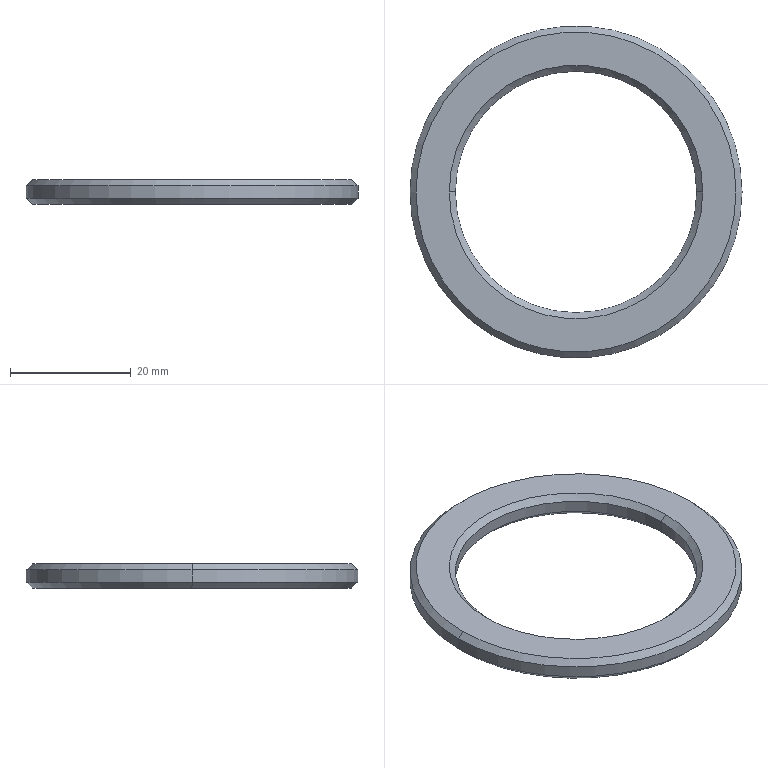Part | STEP file | WASHER_DIA40_1V11 | 1 solid | 14 faces | box 55 x 55 x 4 mm | volume 4178 mm3 | cone 8 | cylinder 4 | plane 2 | commonest cylinder face diameters 40 x2 55 x2
STEP:
#1=CARTESIAN_POINT('',(0.,0.,0.));
#2=DIRECTION('',(0.,0.,1.));
#3=DIRECTION('',(1.,0.,0.));
#4=AXIS2_PLACEMENT_3D('',#1,#2,#3);
#5=CARTESIAN_POINT('',(26.5,0.,4.));
#6=VERTEX_POINT('',#5);
#7=CARTESIAN_POINT('',(-26.5,0.,4.));
#8=VERTEX_POINT('',#7);
#9=CARTESIAN_POINT('',(0.,0.,4.));
#10=DIRECTION('',(0.,0.,1.));
#11=DIRECTION('',(1.,0.,0.));
#12=AXIS2_PLACEMENT_3D('',#9,#10,#11);
#13=CIRCLE('',#12,26.5);
#14=CARTESIAN_POINT('',(0.,0.,4.));
#15=DIRECTION('',(0.,0.,-1.));
#16=DIRECTION('',(-1.,0.,0.));
#17=AXIS2_PLACEMENT_3D('',#14,#15,#16);
#18=CONICAL_SURFACE('',#17,26.5,0.7854);
#19=CARTESIAN_POINT('',(3.142,0.));
#20=DIRECTION('',(-1.,0.));
#21=VECTOR('',#20,1.);
#22=LINE('',#19,#21);
#23=(GEOMETRIC_REPRESENTATION_CONTEXT(2)PARAMETRIC_REPRESENTATION_CONTEXT()REPRESENTATION_CONTEXT('',''));
#24=DEFINITIONAL_REPRESENTATION('',(#22),#23);
#25=PCURVE('',#18,#24);
#26=CARTESIAN_POINT('',(0.,0.,4.));
#27=DIRECTION('',(0.,0.,1.));
#28=DIRECTION('',(1.,0.,0.));
#29=AXIS2_PLACEMENT_3D('',#26,#27,#28);
#30=PLANE('',#29);
#31=CARTESIAN_POINT('',(0.,0.));
#32=DIRECTION('',(1.,0.));
#33=AXIS2_PLACEMENT_2D('',#31,#32);
#34=CIRCLE('',#33,26.5);
#35=(GEOMETRIC_REPRESENTATION_CONTEXT(2)PARAMETRIC_REPRESENTATION_CONTEXT()REPRESENTATION_CONTEXT('',''));
#36=DEFINITIONAL_REPRESENTATION('',(#34),#35);
#37=PCURVE('',#30,#36);
#38=SURFACE_CURVE('',#13,(#25,#37),.PCURVE_S1.);
#39=EDGE_CURVE('',#6,#8,#38,.T.);
#40=ORIENTED_EDGE('',*,*,#39,.F.);
#41=CARTESIAN_POINT('',(27.5,0.,3.));
#42=VERTEX_POINT('',#41);
#43=CARTESIAN_POINT('',(26.5,0.,4.));
#44=DIRECTION('',(0.7071,0.,-0.7071));
#45=VECTOR('',#44,1.);
#46=LINE('',#43,#45);
#47=CARTESIAN_POINT('',(3.142,0.));
#48=DIRECTION('',(0.,1.));
#49=VECTOR('',#48,1.);
#50=LINE('',#47,#49);
#51=(GEOMETRIC_REPRESENTATION_CONTEXT(2)PARAMETRIC_REPRESENTATION_CONTEXT()REPRESENTATION_CONTEXT('',''));
#52=DEFINITIONAL_REPRESENTATION('',(#50),#51);
#53=PCURVE('',#18,#52);
#54=CARTESIAN_POINT('',(0.,0.,4.));
#55=DIRECTION('',(0.,0.,-1.));
#56=DIRECTION('',(-1.,0.,0.));
#57=AXIS2_PLACEMENT_3D('',#54,#55,#56);
#58=CONICAL_SURFACE('',#57,26.5,0.7854);
#59=CARTESIAN_POINT('',(3.142,0.));
#60=DIRECTION('',(0.,1.));
#61=VECTOR('',#60,1.);
#62=LINE('',#59,#61);
#63=(GEOMETRIC_REPRESENTATION_CONTEXT(2)PARAMETRIC_REPRESENTATION_CONTEXT()REPRESENTATION_CONTEXT('',''));
#64=DEFINITIONAL_REPRESENTATION('',(#62),#63);
#65=PCURVE('',#58,#64);
#66=SURFACE_CURVE('',#46,(#53,#65),.PCURVE_S1.);
#67=EDGE_CURVE('',#6,#42,#66,.T.);
#68=ORIENTED_EDGE('',*,*,#67,.T.);
#69=CARTESIAN_POINT('',(-27.5,0.,3.));
#70=VERTEX_POINT('',#69);
#71=CARTESIAN_POINT('',(0.,0.,3.));
#72=DIRECTION('',(0.,0.,-1.));
#73=DIRECTION('',(1.,0.,0.));
#74=AXIS2_PLACEMENT_3D('',#71,#72,#73);
#75=CIRCLE('',#74,27.5);
#76=CARTESIAN_POINT('',(-3.142,1.));
#77=DIRECTION('',(1.,0.));
#78=VECTOR('',#77,1.);
#79=LINE('',#76,#78);
#80=(GEOMETRIC_REPRESENTATION_CONTEXT(2)PARAMETRIC_REPRESENTATION_CONTEXT()REPRESENTATION_CONTEXT('',''));
#81=DEFINITIONAL_REPRESENTATION('',(#79),#80);
#82=PCURVE('',#18,#81);
#83=CARTESIAN_POINT('',(0.,0.,4.));
#84=DIRECTION('',(0.,0.,-1.));
#85=DIRECTION('',(-1.,0.,0.));
#86=AXIS2_PLACEMENT_3D('',#83,#84,#85);
#87=CYLINDRICAL_SURFACE('',#86,27.5);
#88=CARTESIAN_POINT('',(-3.142,1.));
#89=DIRECTION('',(1.,0.));
#90=VECTOR('',#89,1.);
#91=LINE('',#88,#90);
#92=(GEOMETRIC_REPRESENTATION_CONTEXT(2)PARAMETRIC_REPRESENTATION_CONTEXT()REPRESENTATION_CONTEXT('',''));
#93=DEFINITIONAL_REPRESENTATION('',(#91),#92);
#94=PCURVE('',#87,#93);
#95=SURFACE_CURVE('',#75,(#82,#94),.PCURVE_S1.);
#96=EDGE_CURVE('',#70,#42,#95,.T.);
#97=ORIENTED_EDGE('',*,*,#96,.F.);
#98=CARTESIAN_POINT('',(-26.5,0.,4.));
#99=DIRECTION('',(-0.7071,0.,-0.7071));
#100=VECTOR('',#99,1.);
#101=LINE('',#98,#100);
#102=CARTESIAN_POINT('',(0.,0.));
#103=DIRECTION('',(0.,1.));
#104=VECTOR('',#103,1.);
#105=LINE('',#102,#104);
#106=(GEOMETRIC_REPRESENTATION_CONTEXT(2)PARAMETRIC_REPRESENTATION_CONTEXT()REPRESENTATION_CONTEXT('',''));
#107=DEFINITIONAL_REPRESENTATION('',(#105),#106);
#108=PCURVE('',#18,#107);
#109=CARTESIAN_POINT('',(6.283,0.));
#110=DIRECTION('',(0.,1.));
#111=VECTOR('',#110,1.);
#112=LINE('',#109,#111);
#113=(GEOMETRIC_REPRESENTATION_CONTEXT(2)PARAMETRIC_REPRESENTATION_CONTEXT()REPRESENTATION_CONTEXT('',''));
#114=DEFINITIONAL_REPRESENTATION('',(#112),#113);
#115=PCURVE('',#58,#114);
#116=SURFACE_CURVE('',#101,(#108,#115),.PCURVE_S1.);
#117=EDGE_CURVE('',#8,#70,#116,.T.);
#118=ORIENTED_EDGE('',*,*,#117,.F.);
#119=EDGE_LOOP('',(#40,#68,#97,#118));
#120=FACE_BOUND('',#119,.T.);
#121=ADVANCED_FACE('',(#120),#18,.T.);
#122=CARTESIAN_POINT('',(-26.5,0.,0.));
#123=VERTEX_POINT('',#122);
#124=CARTESIAN_POINT('',(26.5,0.,0.));
#125=VERTEX_POINT('',#124);
#126=CARTESIAN_POINT('',(0.,0.,0.));
#127=DIRECTION('',(0.,0.,-1.));
#128=DIRECTION('',(1.,0.,0.));
#129=AXIS2_PLACEMENT_3D('',#126,#127,#128);
#130=CIRCLE('',#129,26.5);
#131=CARTESIAN_POINT('',(0.,0.,1.));
#132=DIRECTION('',(0.,0.,1.));
#133=DIRECTION('',(1.,0.,0.));
#134=AXIS2_PLACEMENT_3D('',#131,#132,#133);
#135=CONICAL_SURFACE('',#134,27.5,0.7854);
#136=CARTESIAN_POINT('',(6.283,-1.));
#137=DIRECTION('',(-1.,0.));
#138=VECTOR('',#137,1.);
#139=LINE('',#136,#138);
#140=(GEOMETRIC_REPRESENTATION_CONTEXT(2)PARAMETRIC_REPRESENTATION_CONTEXT()REPRESENTATION_CONTEXT('',''));
#141=DEFINITIONAL_REPRESENTATION('',(#139),#140);
#142=PCURVE('',#135,#141);
#143=CARTESIAN_POINT('',(0.,0.,0.));
#144=DIRECTION('',(0.,0.,1.));
#145=DIRECTION('',(1.,0.,0.));
#146=AXIS2_PLACEMENT_3D('',#143,#144,#145);
#147=PLANE('',#146);
#148=CARTESIAN_POINT('',(26.5,0.));
#149=CARTESIAN_POINT('',(26.5,-45.899));
#150=CARTESIAN_POINT('',(-13.25,-22.95));
#151=CARTESIAN_POINT('',(-53.,0.));
#152=CARTESIAN_POINT('',(-13.25,22.95));
#153=CARTESIAN_POINT('',(26.5,45.899));
#154=CARTESIAN_POINT('',(26.5,0.));
#155=(BOUNDED_CURVE()B_SPLINE_CURVE(2,(#148,#149,#150,#151,#152,#153,#154),.UNSPECIFIED.,.T.,.F.)B_SPLINE_CURVE_WITH_KNOTS((1,2,2,2,2,1),(-2.094,0.,2.094,4.189,6.283,8.378),.UNSPECIFIED.)CURVE()GEOMETRIC_REPRESENTATION_ITEM()RATIONAL_B_SPLINE_CURVE((1.,0.5,1.,0.5,1.,0.5,1.))REPRESENTATION_ITEM(''));
#156=(GEOMETRIC_REPRESENTATION_CONTEXT(2)PARAMETRIC_REPRESENTATION_CONTEXT()REPRESENTATION_CONTEXT('',''));
#157=DEFINITIONAL_REPRESENTATION('',(#155),#156);
#158=PCURVE('',#147,#157);
#159=SURFACE_CURVE('',#130,(#142,#158),.PCURVE_S1.);
#160=EDGE_CURVE('',#123,#125,#159,.T.);
#161=ORIENTED_EDGE('',*,*,#160,.F.);
#162=CARTESIAN_POINT('',(-27.5,0.,1.));
#163=VERTEX_POINT('',#162);
#164=CARTESIAN_POINT('',(-27.5,0.,1.));
#165=DIRECTION('',(-0.7071,0.,0.7071));
#166=VECTOR('',#165,1.);
#167=LINE('',#164,#166);
#168=CARTESIAN_POINT('',(3.142,0.));
#169=DIRECTION('',(0.,1.));
#170=VECTOR('',#169,1.);
#171=LINE('',#168,#170);
#172=(GEOMETRIC_REPRESENTATION_CONTEXT(2)PARAMETRIC_REPRESENTATION_CONTEXT()REPRESENTATION_CONTEXT('',''));
#173=DEFINITIONAL_REPRESENTATION('',(#171),#172);
#174=PCURVE('',#135,#173);
#175=CARTESIAN_POINT('',(0.,0.,1.));
#176=DIRECTION('',(0.,0.,1.));
#177=DIRECTION('',(1.,0.,0.));
#178=AXIS2_PLACEMENT_3D('',#175,#176,#177);
#179=CONICAL_SURFACE('',#178,27.5,0.7854);
#180=CARTESIAN_POINT('',(3.142,0.));
#181=DIRECTION('',(0.,1.));
#182=VECTOR('',#181,1.);
#183=LINE('',#180,#182);
#184=(GEOMETRIC_REPRESENTATION_CONTEXT(2)PARAMETRIC_REPRESENTATION_CONTEXT()REPRESENTATION_CONTEXT('',''));
#185=DEFINITIONAL_REPRESENTATION('',(#183),#184);
#186=PCURVE('',#179,#185);
#187=SURFACE_CURVE('',#167,(#174,#186),.PCURVE_S1.);
#188=EDGE_CURVE('',#123,#163,#187,.T.);
#189=ORIENTED_EDGE('',*,*,#188,.T.);
#190=CARTESIAN_POINT('',(27.5,0.,1.));
#191=VERTEX_POINT('',#190);
#192=CARTESIAN_POINT('',(0.,0.,1.));
#193=DIRECTION('',(0.,0.,1.));
#194=DIRECTION('',(1.,0.,0.));
#195=AXIS2_PLACEMENT_3D('',#192,#193,#194);
#196=CIRCLE('',#195,27.5);
#197=CARTESIAN_POINT('',(0.,0.));
#198=DIRECTION('',(1.,0.));
#199=VECTOR('',#198,1.);
#200=LINE('',#197,#199);
#201=(GEOMETRIC_REPRESENTATION_CONTEXT(2)PARAMETRIC_REPRESENTATION_CONTEXT()REPRESENTATION_CONTEXT('',''));
#202=DEFINITIONAL_REPRESENTATION('',(#200),#201);
#203=PCURVE('',#135,#202);
#204=CARTESIAN_POINT('',(3.142,3.));
#205=DIRECTION('',(-1.,0.));
#206=VECTOR('',#205,1.);
#207=LINE('',#204,#206);
#208=(GEOMETRIC_REPRESENTATION_CONTEXT(2)PARAMETRIC_REPRESENTATION_CONTEXT()REPRESENTATION_CONTEXT('',''));
#209=DEFINITIONAL_REPRESENTATION('',(#207),#208);
#210=PCURVE('',#87,#209);
#211=SURFACE_CURVE('',#196,(#203,#210),.PCURVE_S1.);
#212=EDGE_CURVE('',#191,#163,#211,.T.);
#213=ORIENTED_EDGE('',*,*,#212,.F.);
#214=CARTESIAN_POINT('',(27.5,0.,1.));
#215=DIRECTION('',(0.7071,0.,0.7071));
#216=VECTOR('',#215,1.);
#217=LINE('',#214,#216);
#218=CARTESIAN_POINT('',(0.,0.));
#219=DIRECTION('',(0.,1.));
#220=VECTOR('',#219,1.);
#221=LINE('',#218,#220);
#222=(GEOMETRIC_REPRESENTATION_CONTEXT(2)PARAMETRIC_REPRESENTATION_CONTEXT()REPRESENTATION_CONTEXT('',''));
#223=DEFINITIONAL_REPRESENTATION('',(#221),#222);
#224=PCURVE('',#135,#223);
#225=CARTESIAN_POINT('',(6.283,0.));
#226=DIRECTION('',(0.,1.));
#227=VECTOR('',#226,1.);
#228=LINE('',#225,#227);
#229=(GEOMETRIC_REPRESENTATION_CONTEXT(2)PARAMETRIC_REPRESENTATION_CONTEXT()REPRESENTATION_CONTEXT('',''));
#230=DEFINITIONAL_REPRESENTATION('',(#228),#229);
#231=PCURVE('',#179,#230);
#232=SURFACE_CURVE('',#217,(#224,#231),.PCURVE_S1.);
#233=EDGE_CURVE('',#125,#191,#232,.T.);
#234=ORIENTED_EDGE('',*,*,#233,.F.);
#235=EDGE_LOOP('',(#161,#189,#213,#234));
#236=FACE_BOUND('',#235,.T.);
#237=ADVANCED_FACE('',(#236),#135,.T.);
#238=CARTESIAN_POINT('',(20.,0.,3.));
#239=VERTEX_POINT('',#238);
#240=CARTESIAN_POINT('',(21.,0.,4.));
#241=VERTEX_POINT('',#240);
#242=CARTESIAN_POINT('',(20.,0.,3.));
#243=DIRECTION('',(0.7071,0.,0.7071));
#244=VECTOR('',#243,1.);
#245=LINE('',#242,#244);
#246=CARTESIAN_POINT('',(0.,0.,3.));
#247=DIRECTION('',(0.,0.,1.));
#248=DIRECTION('',(1.,0.,0.));
#249=AXIS2_PLACEMENT_3D('',#246,#247,#248);
#250=CONICAL_SURFACE('',#249,20.,0.7854);
#251=CARTESIAN_POINT('',(6.283,0.));
#252=DIRECTION('',(0.,1.));
#253=VECTOR('',#252,1.);
#254=LINE('',#251,#253);
#255=(GEOMETRIC_REPRESENTATION_CONTEXT(2)PARAMETRIC_REPRESENTATION_CONTEXT()REPRESENTATION_CONTEXT('',''));
#256=DEFINITIONAL_REPRESENTATION('',(#254),#255);
#257=PCURVE('',#250,#256);
#258=CARTESIAN_POINT('',(0.,0.,3.));
#259=DIRECTION('',(0.,0.,1.));
#260=DIRECTION('',(1.,0.,0.));
#261=AXIS2_PLACEMENT_3D('',#258,#259,#260);
#262=CONICAL_SURFACE('',#261,20.,0.7854);
#263=CARTESIAN_POINT('',(0.,0.));
#264=DIRECTION('',(0.,1.));
#265=VECTOR('',#264,1.);
#266=LINE('',#263,#265);
#267=(GEOMETRIC_REPRESENTATION_CONTEXT(2)PARAMETRIC_REPRESENTATION_CONTEXT()REPRESENTATION_CONTEXT('',''));
#268=DEFINITIONAL_REPRESENTATION('',(#266),#267);
#269=PCURVE('',#262,#268);
#270=SURFACE_CURVE('',#245,(#257,#269),.PCURVE_S1.);
#271=EDGE_CURVE('',#239,#241,#270,.T.);
#272=ORIENTED_EDGE('',*,*,#271,.T.);
#273=CARTESIAN_POINT('',(-21.,0.,4.));
#274=VERTEX_POINT('',#273);
#275=CARTESIAN_POINT('',(0.,0.,4.));
#276=DIRECTION('',(0.,0.,-1.));
#277=DIRECTION('',(1.,0.,0.));
#278=AXIS2_PLACEMENT_3D('',#275,#276,#277);
#279=CIRCLE('',#278,21.);
#280=CARTESIAN_POINT('',(6.283,1.));
#281=DIRECTION('',(-1.,0.));
#282=VECTOR('',#281,1.);
#283=LINE('',#280,#282);
#284=(GEOMETRIC_REPRESENTATION_CONTEXT(2)PARAMETRIC_REPRESENTATION_CONTEXT()REPRESENTATION_CONTEXT('',''));
#285=DEFINITIONAL_REPRESENTATION('',(#283),#284);
#286=PCURVE('',#250,#285);
#287=CARTESIAN_POINT('',(21.,0.));
#288=CARTESIAN_POINT('',(21.,-36.373));
#289=CARTESIAN_POINT('',(-10.5,-18.187));
#290=CARTESIAN_POINT('',(-42.,0.));
#291=CARTESIAN_POINT('',(-10.5,18.187));
#292=CARTESIAN_POINT('',(21.,36.373));
#293=CARTESIAN_POINT('',(21.,0.));
#294=(BOUNDED_CURVE()B_SPLINE_CURVE(2,(#287,#288,#289,#290,#291,#292,#293),.UNSPECIFIED.,.T.,.F.)B_SPLINE_CURVE_WITH_KNOTS((1,2,2,2,2,1),(-2.094,0.,2.094,4.189,6.283,8.378),.UNSPECIFIED.)CURVE()GEOMETRIC_REPRESENTATION_ITEM()RATIONAL_B_SPLINE_CURVE((1.,0.5,1.,0.5,1.,0.5,1.))REPRESENTATION_ITEM(''));
#295=(GEOMETRIC_REPRESENTATION_CONTEXT(2)PARAMETRIC_REPRESENTATION_CONTEXT()REPRESENTATION_CONTEXT('',''));
#296=DEFINITIONAL_REPRESENTATION('',(#294),#295);
#297=PCURVE('',#30,#296);
#298=SURFACE_CURVE('',#279,(#286,#297),.PCURVE_S1.);
#299=EDGE_CURVE('',#241,#274,#298,.T.);
#300=ORIENTED_EDGE('',*,*,#299,.T.);
#301=CARTESIAN_POINT('',(-20.,0.,3.));
#302=VERTEX_POINT('',#301);
#303=CARTESIAN_POINT('',(-20.,0.,3.));
#304=DIRECTION('',(-0.7071,0.,0.7071));
#305=VECTOR('',#304,1.);
#306=LINE('',#303,#305);
#307=CARTESIAN_POINT('',(3.142,0.));
#308=DIRECTION('',(0.,1.));
#309=VECTOR('',#308,1.);
#310=LINE('',#307,#309);
#311=(GEOMETRIC_REPRESENTATION_CONTEXT(2)PARAMETRIC_REPRESENTATION_CONTEXT()REPRESENTATION_CONTEXT('',''));
#312=DEFINITIONAL_REPRESENTATION('',(#310),#311);
#313=PCURVE('',#250,#312);
#314=CARTESIAN_POINT('',(3.142,0.));
#315=DIRECTION('',(0.,1.));
#316=VECTOR('',#315,1.);
#317=LINE('',#314,#316);
#318=(GEOMETRIC_REPRESENTATION_CONTEXT(2)PARAMETRIC_REPRESENTATION_CONTEXT()REPRESENTATION_CONTEXT('',''));
#319=DEFINITIONAL_REPRESENTATION('',(#317),#318);
#320=PCURVE('',#262,#319);
#321=SURFACE_CURVE('',#306,(#313,#320),.PCURVE_S1.);
#322=EDGE_CURVE('',#302,#274,#321,.T.);
#323=ORIENTED_EDGE('',*,*,#322,.F.);
#324=CARTESIAN_POINT('',(0.,0.,3.));
#325=DIRECTION('',(0.,0.,1.));
#326=DIRECTION('',(1.,0.,0.));
#327=AXIS2_PLACEMENT_3D('',#324,#325,#326);
#328=CIRCLE('',#327,20.);
#329=CARTESIAN_POINT('',(0.,0.));
#330=DIRECTION('',(1.,0.));
#331=VECTOR('',#330,1.);
#332=LINE('',#329,#331);
#333=(GEOMETRIC_REPRESENTATION_CONTEXT(2)PARAMETRIC_REPRESENTATION_CONTEXT()REPRESENTATION_CONTEXT('',''));
#334=DEFINITIONAL_REPRESENTATION('',(#332),#333);
#335=PCURVE('',#250,#334);
#336=CARTESIAN_POINT('',(0.,0.,4.));
#337=DIRECTION('',(0.,0.,-1.));
#338=DIRECTION('',(-1.,0.,0.));
#339=AXIS2_PLACEMENT_3D('',#336,#337,#338);
#340=CYLINDRICAL_SURFACE('',#339,20.);
#341=CARTESIAN_POINT('',(9.425,1.));
#342=DIRECTION('',(-1.,0.));
#343=VECTOR('',#342,1.);
#344=LINE('',#341,#343);
#345=(GEOMETRIC_REPRESENTATION_CONTEXT(2)PARAMETRIC_REPRESENTATION_CONTEXT()REPRESENTATION_CONTEXT('',''));
#346=DEFINITIONAL_REPRESENTATION('',(#344),#345);
#347=PCURVE('',#340,#346);
#348=SURFACE_CURVE('',#328,(#335,#347),.PCURVE_S1.);
#349=EDGE_CURVE('',#302,#239,#348,.T.);
#350=ORIENTED_EDGE('',*,*,#349,.T.);
#351=EDGE_LOOP('',(#272,#300,#323,#350));
#352=FACE_BOUND('',#351,.F.);
#353=ADVANCED_FACE('',(#352),#250,.F.);
#354=CARTESIAN_POINT('',(-20.,0.,1.));
#355=VERTEX_POINT('',#354);
#356=CARTESIAN_POINT('',(-21.,0.,0.));
#357=VERTEX_POINT('',#356);
#358=CARTESIAN_POINT('',(-21.,0.,0.));
#359=DIRECTION('',(-0.7071,0.,-0.7071));
#360=VECTOR('',#359,1.);
#361=LINE('',#358,#360);
#362=CARTESIAN_POINT('',(0.,0.,0.));
#363=DIRECTION('',(0.,0.,-1.));
#364=DIRECTION('',(-1.,0.,0.));
#365=AXIS2_PLACEMENT_3D('',#362,#363,#364);
#366=CONICAL_SURFACE('',#365,21.,0.7854);
#367=CARTESIAN_POINT('',(6.283,0.));
#368=DIRECTION('',(0.,1.));
#369=VECTOR('',#368,1.);
#370=LINE('',#367,#369);
#371=(GEOMETRIC_REPRESENTATION_CONTEXT(2)PARAMETRIC_REPRESENTATION_CONTEXT()REPRESENTATION_CONTEXT('',''));
#372=DEFINITIONAL_REPRESENTATION('',(#370),#371);
#373=PCURVE('',#366,#372);
#374=CARTESIAN_POINT('',(0.,0.,0.));
#375=DIRECTION('',(0.,0.,-1.));
#376=DIRECTION('',(-1.,0.,0.));
#377=AXIS2_PLACEMENT_3D('',#374,#375,#376);
#378=CONICAL_SURFACE('',#377,21.,0.7854);
#379=CARTESIAN_POINT('',(0.,0.));
#380=DIRECTION('',(0.,1.));
#381=VECTOR('',#380,1.);
#382=LINE('',#379,#381);
#383=(GEOMETRIC_REPRESENTATION_CONTEXT(2)PARAMETRIC_REPRESENTATION_CONTEXT()REPRESENTATION_CONTEXT('',''));
#384=DEFINITIONAL_REPRESENTATION('',(#382),#383);
#385=PCURVE('',#378,#384);
#386=SURFACE_CURVE('',#361,(#373,#385),.PCURVE_S1.);
#387=EDGE_CURVE('',#355,#357,#386,.T.);
#388=ORIENTED_EDGE('',*,*,#387,.T.);
#389=CARTESIAN_POINT('',(21.,0.,0.));
#390=VERTEX_POINT('',#389);
#391=CARTESIAN_POINT('',(0.,0.,0.));
#392=DIRECTION('',(0.,0.,1.));
#393=DIRECTION('',(1.,0.,0.));
#394=AXIS2_PLACEMENT_3D('',#391,#392,#393);
#395=CIRCLE('',#394,21.);
#396=CARTESIAN_POINT('',(9.425,0.));
#397=DIRECTION('',(-1.,0.));
#398=VECTOR('',#397,1.);
#399=LINE('',#396,#398);
#400=(GEOMETRIC_REPRESENTATION_CONTEXT(2)PARAMETRIC_REPRESENTATION_CONTEXT()REPRESENTATION_CONTEXT('',''));
#401=DEFINITIONAL_REPRESENTATION('',(#399),#400);
#402=PCURVE('',#366,#401);
#403=CARTESIAN_POINT('',(0.,0.));
#404=DIRECTION('',(1.,0.));
#405=AXIS2_PLACEMENT_2D('',#403,#404);
#406=CIRCLE('',#405,21.);
#407=(GEOMETRIC_REPRESENTATION_CONTEXT(2)PARAMETRIC_REPRESENTATION_CONTEXT()REPRESENTATION_CONTEXT('',''));
#408=DEFINITIONAL_REPRESENTATION('',(#406),#407);
#409=PCURVE('',#147,#408);
#410=SURFACE_CURVE('',#395,(#402,#409),.PCURVE_S1.);
#411=EDGE_CURVE('',#357,#390,#410,.T.);
#412=ORIENTED_EDGE('',*,*,#411,.T.);
#413=CARTESIAN_POINT('',(20.,0.,1.));
#414=VERTEX_POINT('',#413);
#415=CARTESIAN_POINT('',(21.,0.,0.));
#416=DIRECTION('',(0.7071,0.,-0.7071));
#417=VECTOR('',#416,1.);
#418=LINE('',#415,#417);
#419=CARTESIAN_POINT('',(3.142,0.));
#420=DIRECTION('',(0.,1.));
#421=VECTOR('',#420,1.);
#422=LINE('',#419,#421);
#423=(GEOMETRIC_REPRESENTATION_CONTEXT(2)PARAMETRIC_REPRESENTATION_CONTEXT()REPRESENTATION_CONTEXT('',''));
#424=DEFINITIONAL_REPRESENTATION('',(#422),#423);
#425=PCURVE('',#366,#424);
#426=CARTESIAN_POINT('',(3.142,0.));
#427=DIRECTION('',(0.,1.));
#428=VECTOR('',#427,1.);
#429=LINE('',#426,#428);
#430=(GEOMETRIC_REPRESENTATION_CONTEXT(2)PARAMETRIC_REPRESENTATION_CONTEXT()REPRESENTATION_CONTEXT('',''));
#431=DEFINITIONAL_REPRESENTATION('',(#429),#430);
#432=PCURVE('',#378,#431);
#433=SURFACE_CURVE('',#418,(#425,#432),.PCURVE_S1.);
#434=EDGE_CURVE('',#414,#390,#433,.T.);
#435=ORIENTED_EDGE('',*,*,#434,.F.);
#436=CARTESIAN_POINT('',(0.,0.,1.));
#437=DIRECTION('',(0.,0.,-1.));
#438=DIRECTION('',(1.,0.,0.));
#439=AXIS2_PLACEMENT_3D('',#436,#437,#438);
#440=CIRCLE('',#439,20.);
#441=CARTESIAN_POINT('',(3.142,-1.));
#442=DIRECTION('',(1.,0.));
#443=VECTOR('',#442,1.);
#444=LINE('',#441,#443);
#445=(GEOMETRIC_REPRESENTATION_CONTEXT(2)PARAMETRIC_REPRESENTATION_CONTEXT()REPRESENTATION_CONTEXT('',''));
#446=DEFINITIONAL_REPRESENTATION('',(#444),#445);
#447=PCURVE('',#366,#446);
#448=CARTESIAN_POINT('',(3.142,3.));
#449=DIRECTION('',(1.,0.));
#450=VECTOR('',#449,1.);
#451=LINE('',#448,#450);
#452=(GEOMETRIC_REPRESENTATION_CONTEXT(2)PARAMETRIC_REPRESENTATION_CONTEXT()REPRESENTATION_CONTEXT('',''));
#453=DEFINITIONAL_REPRESENTATION('',(#451),#452);
#454=PCURVE('',#340,#453);
#455=SURFACE_CURVE('',#440,(#447,#454),.PCURVE_S1.);
#456=EDGE_CURVE('',#414,#355,#455,.T.);
#457=ORIENTED_EDGE('',*,*,#456,.T.);
#458=EDGE_LOOP('',(#388,#412,#435,#457));
#459=FACE_BOUND('',#458,.F.);
#460=ADVANCED_FACE('',(#459),#366,.F.);
#461=CARTESIAN_POINT('',(-20.,0.,4.));
#462=DIRECTION('',(0.,0.,-1.));
#463=VECTOR('',#462,1.);
#464=LINE('',#461,#463);
#465=CARTESIAN_POINT('',(6.283,0.));
#466=DIRECTION('',(0.,1.));
#467=VECTOR('',#466,1.);
#468=LINE('',#465,#467);
#469=(GEOMETRIC_REPRESENTATION_CONTEXT(2)PARAMETRIC_REPRESENTATION_CONTEXT()REPRESENTATION_CONTEXT('',''));
#470=DEFINITIONAL_REPRESENTATION('',(#468),#469);
#471=PCURVE('',#340,#470);
#472=CARTESIAN_POINT('',(0.,0.,4.));
#473=DIRECTION('',(0.,0.,-1.));
#474=DIRECTION('',(-1.,0.,0.));
#475=AXIS2_PLACEMENT_3D('',#472,#473,#474);
#476=CYLINDRICAL_SURFACE('',#475,20.);
#477=CARTESIAN_POINT('',(0.,0.));
#478=DIRECTION('',(0.,1.));
#479=VECTOR('',#478,1.);
#480=LINE('',#477,#479);
#481=(GEOMETRIC_REPRESENTATION_CONTEXT(2)PARAMETRIC_REPRESENTATION_CONTEXT()REPRESENTATION_CONTEXT('',''));
#482=DEFINITIONAL_REPRESENTATION('',(#480),#481);
#483=PCURVE('',#476,#482);
#484=SURFACE_CURVE('',#464,(#471,#483),.PCURVE_S1.);
#485=EDGE_CURVE('',#302,#355,#484,.T.);
#486=ORIENTED_EDGE('',*,*,#485,.T.);
#487=ORIENTED_EDGE('',*,*,#456,.F.);
#488=CARTESIAN_POINT('',(20.,0.,4.));
#489=DIRECTION('',(0.,0.,-1.));
#490=VECTOR('',#489,1.);
#491=LINE('',#488,#490);
#492=CARTESIAN_POINT('',(3.142,0.));
#493=DIRECTION('',(0.,1.));
#494=VECTOR('',#493,1.);
#495=LINE('',#492,#494);
#496=(GEOMETRIC_REPRESENTATION_CONTEXT(2)PARAMETRIC_REPRESENTATION_CONTEXT()REPRESENTATION_CONTEXT('',''));
#497=DEFINITIONAL_REPRESENTATION('',(#495),#496);
#498=PCURVE('',#340,#497);
#499=CARTESIAN_POINT('',(3.142,0.));
#500=DIRECTION('',(0.,1.));
#501=VECTOR('',#500,1.);
#502=LINE('',#499,#501);
#503=(GEOMETRIC_REPRESENTATION_CONTEXT(2)PARAMETRIC_REPRESENTATION_CONTEXT()REPRESENTATION_CONTEXT('',''));
#504=DEFINITIONAL_REPRESENTATION('',(#502),#503);
#505=PCURVE('',#476,#504);
#506=SURFACE_CURVE('',#491,(#498,#505),.PCURVE_S1.);
#507=EDGE_CURVE('',#239,#414,#506,.T.);
#508=ORIENTED_EDGE('',*,*,#507,.F.);
#509=ORIENTED_EDGE('',*,*,#349,.F.);
#510=EDGE_LOOP('',(#486,#487,#508,#509));
#511=FACE_BOUND('',#510,.F.);
#512=ADVANCED_FACE('',(#511),#340,.F.);
#513=ORIENTED_EDGE('',*,*,#96,.T.);
#514=CARTESIAN_POINT('',(27.5,0.,4.));
#515=DIRECTION('',(0.,0.,-1.));
#516=VECTOR('',#515,1.);
#517=LINE('',#514,#516);
#518=CARTESIAN_POINT('',(3.142,0.));
#519=DIRECTION('',(0.,1.));
#520=VECTOR('',#519,1.);
#521=LINE('',#518,#520);
#522=(GEOMETRIC_REPRESENTATION_CONTEXT(2)PARAMETRIC_REPRESENTATION_CONTEXT()REPRESENTATION_CONTEXT('',''));
#523=DEFINITIONAL_REPRESENTATION('',(#521),#522);
#524=PCURVE('',#87,#523);
#525=CARTESIAN_POINT('',(0.,0.,4.));
#526=DIRECTION('',(0.,0.,-1.));
#527=DIRECTION('',(-1.,0.,0.));
#528=AXIS2_PLACEMENT_3D('',#525,#526,#527);
#529=CYLINDRICAL_SURFACE('',#528,27.5);
#530=CARTESIAN_POINT('',(3.142,0.));
#531=DIRECTION('',(0.,1.));
#532=VECTOR('',#531,1.);
#533=LINE('',#530,#532);
#534=(GEOMETRIC_REPRESENTATION_CONTEXT(2)PARAMETRIC_REPRESENTATION_CONTEXT()REPRESENTATION_CONTEXT('',''));
#535=DEFINITIONAL_REPRESENTATION('',(#533),#534);
#536=PCURVE('',#529,#535);
#537=SURFACE_CURVE('',#517,(#524,#536),.PCURVE_S1.);
#538=EDGE_CURVE('',#42,#191,#537,.T.);
#539=ORIENTED_EDGE('',*,*,#538,.T.);
#540=ORIENTED_EDGE('',*,*,#212,.T.);
#541=CARTESIAN_POINT('',(-27.5,0.,4.));
#542=DIRECTION('',(0.,0.,-1.));
#543=VECTOR('',#542,1.);
#544=LINE('',#541,#543);
#545=CARTESIAN_POINT('',(0.,0.));
#546=DIRECTION('',(0.,1.));
#547=VECTOR('',#546,1.);
#548=LINE('',#545,#547);
#549=(GEOMETRIC_REPRESENTATION_CONTEXT(2)PARAMETRIC_REPRESENTATION_CONTEXT()REPRESENTATION_CONTEXT('',''));
#550=DEFINITIONAL_REPRESENTATION('',(#548),#549);
#551=PCURVE('',#87,#550);
#552=CARTESIAN_POINT('',(6.283,0.));
#553=DIRECTION('',(0.,1.));
#554=VECTOR('',#553,1.);
#555=LINE('',#552,#554);
#556=(GEOMETRIC_REPRESENTATION_CONTEXT(2)PARAMETRIC_REPRESENTATION_CONTEXT()REPRESENTATION_CONTEXT('',''));
#557=DEFINITIONAL_REPRESENTATION('',(#555),#556);
#558=PCURVE('',#529,#557);
#559=SURFACE_CURVE('',#544,(#551,#558),.PCURVE_S1.);
#560=EDGE_CURVE('',#70,#163,#559,.T.);
#561=ORIENTED_EDGE('',*,*,#560,.F.);
#562=EDGE_LOOP('',(#513,#539,#540,#561));
#563=FACE_BOUND('',#562,.T.);
#564=ADVANCED_FACE('',(#563),#87,.T.);
#565=CARTESIAN_POINT('',(0.,0.,4.));
#566=DIRECTION('',(0.,0.,1.));
#567=DIRECTION('',(1.,0.,0.));
#568=AXIS2_PLACEMENT_3D('',#565,#566,#567);
#569=CIRCLE('',#568,26.5);
#570=CARTESIAN_POINT('',(0.,0.));
#571=DIRECTION('',(1.,0.));
#572=AXIS2_PLACEMENT_2D('',#570,#571);
#573=CIRCLE('',#572,26.5);
#574=(GEOMETRIC_REPRESENTATION_CONTEXT(2)PARAMETRIC_REPRESENTATION_CONTEXT()REPRESENTATION_CONTEXT('',''));
#575=DEFINITIONAL_REPRESENTATION('',(#573),#574);
#576=PCURVE('',#30,#575);
#577=CARTESIAN_POINT('',(9.425,0.));
#578=DIRECTION('',(-1.,0.));
#579=VECTOR('',#578,1.);
#580=LINE('',#577,#579);
#581=(GEOMETRIC_REPRESENTATION_CONTEXT(2)PARAMETRIC_REPRESENTATION_CONTEXT()REPRESENTATION_CONTEXT('',''));
#582=DEFINITIONAL_REPRESENTATION('',(#580),#581);
#583=PCURVE('',#58,#582);
#584=SURFACE_CURVE('',#569,(#576,#583),.PCURVE_S1.);
#585=EDGE_CURVE('',#8,#6,#584,.T.);
#586=ORIENTED_EDGE('',*,*,#585,.T.);
#587=ORIENTED_EDGE('',*,*,#39,.T.);
#588=EDGE_LOOP('',(#586,#587));
#589=FACE_BOUND('',#588,.T.);
#590=ORIENTED_EDGE('',*,*,#299,.T.);
#591=CARTESIAN_POINT('',(0.,0.,4.));
#592=DIRECTION('',(0.,0.,-1.));
#593=DIRECTION('',(1.,0.,0.));
#594=AXIS2_PLACEMENT_3D('',#591,#592,#593);
#595=CIRCLE('',#594,21.);
#596=CARTESIAN_POINT('',(21.,0.));
#597=CARTESIAN_POINT('',(21.,-36.373));
#598=CARTESIAN_POINT('',(-10.5,-18.187));
#599=CARTESIAN_POINT('',(-42.,0.));
#600=CARTESIAN_POINT('',(-10.5,18.187));
#601=CARTESIAN_POINT('',(21.,36.373));
#602=CARTESIAN_POINT('',(21.,0.));
#603=(BOUNDED_CURVE()B_SPLINE_CURVE(2,(#596,#597,#598,#599,#600,#601,#602),.UNSPECIFIED.,.T.,.F.)B_SPLINE_CURVE_WITH_KNOTS((1,2,2,2,2,1),(-2.094,0.,2.094,4.189,6.283,8.378),.UNSPECIFIED.)CURVE()GEOMETRIC_REPRESENTATION_ITEM()RATIONAL_B_SPLINE_CURVE((1.,0.5,1.,0.5,1.,0.5,1.))REPRESENTATION_ITEM(''));
#604=(GEOMETRIC_REPRESENTATION_CONTEXT(2)PARAMETRIC_REPRESENTATION_CONTEXT()REPRESENTATION_CONTEXT('',''));
#605=DEFINITIONAL_REPRESENTATION('',(#603),#604);
#606=PCURVE('',#30,#605);
#607=CARTESIAN_POINT('',(6.283,1.));
#608=DIRECTION('',(-1.,0.));
#609=VECTOR('',#608,1.);
#610=LINE('',#607,#609);
#611=(GEOMETRIC_REPRESENTATION_CONTEXT(2)PARAMETRIC_REPRESENTATION_CONTEXT()REPRESENTATION_CONTEXT('',''));
#612=DEFINITIONAL_REPRESENTATION('',(#610),#611);
#613=PCURVE('',#262,#612);
#614=SURFACE_CURVE('',#595,(#606,#613),.PCURVE_S1.);
#615=EDGE_CURVE('',#274,#241,#614,.T.);
#616=ORIENTED_EDGE('',*,*,#615,.T.);
#617=EDGE_LOOP('',(#590,#616));
#618=FACE_BOUND('',#617,.T.);
#619=ADVANCED_FACE('',(#589,#618),#30,.T.);
#620=CARTESIAN_POINT('',(0.,0.,0.));
#621=DIRECTION('',(0.,0.,-1.));
#622=DIRECTION('',(1.,0.,0.));
#623=AXIS2_PLACEMENT_3D('',#620,#621,#622);
#624=CIRCLE('',#623,26.5);
#625=CARTESIAN_POINT('',(26.5,0.));
#626=CARTESIAN_POINT('',(26.5,-45.899));
#627=CARTESIAN_POINT('',(-13.25,-22.95));
#628=CARTESIAN_POINT('',(-53.,0.));
#629=CARTESIAN_POINT('',(-13.25,22.95));
#630=CARTESIAN_POINT('',(26.5,45.899));
#631=CARTESIAN_POINT('',(26.5,0.));
#632=(BOUNDED_CURVE()B_SPLINE_CURVE(2,(#625,#626,#627,#628,#629,#630,#631),.UNSPECIFIED.,.T.,.F.)B_SPLINE_CURVE_WITH_KNOTS((1,2,2,2,2,1),(-2.094,0.,2.094,4.189,6.283,8.378),.UNSPECIFIED.)CURVE()GEOMETRIC_REPRESENTATION_ITEM()RATIONAL_B_SPLINE_CURVE((1.,0.5,1.,0.5,1.,0.5,1.))REPRESENTATION_ITEM(''));
#633=(GEOMETRIC_REPRESENTATION_CONTEXT(2)PARAMETRIC_REPRESENTATION_CONTEXT()REPRESENTATION_CONTEXT('',''));
#634=DEFINITIONAL_REPRESENTATION('',(#632),#633);
#635=PCURVE('',#147,#634);
#636=CARTESIAN_POINT('',(6.283,-1.));
#637=DIRECTION('',(-1.,0.));
#638=VECTOR('',#637,1.);
#639=LINE('',#636,#638);
#640=(GEOMETRIC_REPRESENTATION_CONTEXT(2)PARAMETRIC_REPRESENTATION_CONTEXT()REPRESENTATION_CONTEXT('',''));
#641=DEFINITIONAL_REPRESENTATION('',(#639),#640);
#642=PCURVE('',#179,#641);
#643=SURFACE_CURVE('',#624,(#635,#642),.PCURVE_S1.);
#644=EDGE_CURVE('',#125,#123,#643,.T.);
#645=ORIENTED_EDGE('',*,*,#644,.T.);
#646=ORIENTED_EDGE('',*,*,#160,.T.);
#647=EDGE_LOOP('',(#645,#646));
#648=FACE_BOUND('',#647,.T.);
#649=ORIENTED_EDGE('',*,*,#411,.T.);
#650=CARTESIAN_POINT('',(0.,0.,0.));
#651=DIRECTION('',(0.,0.,1.));
#652=DIRECTION('',(1.,0.,0.));
#653=AXIS2_PLACEMENT_3D('',#650,#651,#652);
#654=CIRCLE('',#653,21.);
#655=CARTESIAN_POINT('',(0.,0.));
#656=DIRECTION('',(1.,0.));
#657=AXIS2_PLACEMENT_2D('',#655,#656);
#658=CIRCLE('',#657,21.);
#659=(GEOMETRIC_REPRESENTATION_CONTEXT(2)PARAMETRIC_REPRESENTATION_CONTEXT()REPRESENTATION_CONTEXT('',''));
#660=DEFINITIONAL_REPRESENTATION('',(#658),#659);
#661=PCURVE('',#147,#660);
#662=CARTESIAN_POINT('',(3.142,0.));
#663=DIRECTION('',(-1.,0.));
#664=VECTOR('',#663,1.);
#665=LINE('',#662,#664);
#666=(GEOMETRIC_REPRESENTATION_CONTEXT(2)PARAMETRIC_REPRESENTATION_CONTEXT()REPRESENTATION_CONTEXT('',''));
#667=DEFINITIONAL_REPRESENTATION('',(#665),#666);
#668=PCURVE('',#378,#667);
#669=SURFACE_CURVE('',#654,(#661,#668),.PCURVE_S1.);
#670=EDGE_CURVE('',#390,#357,#669,.T.);
#671=ORIENTED_EDGE('',*,*,#670,.T.);
#672=EDGE_LOOP('',(#649,#671));
#673=FACE_BOUND('',#672,.T.);
#674=ADVANCED_FACE('',(#648,#673),#147,.F.);
#675=ORIENTED_EDGE('',*,*,#538,.F.);
#676=CARTESIAN_POINT('',(0.,0.,3.));
#677=DIRECTION('',(0.,0.,-1.));
#678=DIRECTION('',(1.,0.,0.));
#679=AXIS2_PLACEMENT_3D('',#676,#677,#678);
#680=CIRCLE('',#679,27.5);
#681=CARTESIAN_POINT('',(3.142,1.));
#682=DIRECTION('',(1.,0.));
#683=VECTOR('',#682,1.);
#684=LINE('',#681,#683);
#685=(GEOMETRIC_REPRESENTATION_CONTEXT(2)PARAMETRIC_REPRESENTATION_CONTEXT()REPRESENTATION_CONTEXT('',''));
#686=DEFINITIONAL_REPRESENTATION('',(#684),#685);
#687=PCURVE('',#529,#686);
#688=CARTESIAN_POINT('',(3.142,1.));
#689=DIRECTION('',(1.,0.));
#690=VECTOR('',#689,1.);
#691=LINE('',#688,#690);
#692=(GEOMETRIC_REPRESENTATION_CONTEXT(2)PARAMETRIC_REPRESENTATION_CONTEXT()REPRESENTATION_CONTEXT('',''));
#693=DEFINITIONAL_REPRESENTATION('',(#691),#692);
#694=PCURVE('',#58,#693);
#695=SURFACE_CURVE('',#680,(#687,#694),.PCURVE_S1.);
#696=EDGE_CURVE('',#42,#70,#695,.T.);
#697=ORIENTED_EDGE('',*,*,#696,.T.);
#698=ORIENTED_EDGE('',*,*,#560,.T.);
#699=CARTESIAN_POINT('',(0.,0.,1.));
#700=DIRECTION('',(0.,0.,1.));
#701=DIRECTION('',(1.,0.,0.));
#702=AXIS2_PLACEMENT_3D('',#699,#700,#701);
#703=CIRCLE('',#702,27.5);
#704=CARTESIAN_POINT('',(9.425,3.));
#705=DIRECTION('',(-1.,0.));
#706=VECTOR('',#705,1.);
#707=LINE('',#704,#706);
#708=(GEOMETRIC_REPRESENTATION_CONTEXT(2)PARAMETRIC_REPRESENTATION_CONTEXT()REPRESENTATION_CONTEXT('',''));
#709=DEFINITIONAL_REPRESENTATION('',(#707),#708);
#710=PCURVE('',#529,#709);
#711=CARTESIAN_POINT('',(0.,0.));
#712=DIRECTION('',(1.,0.));
#713=VECTOR('',#712,1.);
#714=LINE('',#711,#713);
#715=(GEOMETRIC_REPRESENTATION_CONTEXT(2)PARAMETRIC_REPRESENTATION_CONTEXT()REPRESENTATION_CONTEXT('',''));
#716=DEFINITIONAL_REPRESENTATION('',(#714),#715);
#717=PCURVE('',#179,#716);
#718=SURFACE_CURVE('',#703,(#710,#717),.PCURVE_S1.);
#719=EDGE_CURVE('',#163,#191,#718,.T.);
#720=ORIENTED_EDGE('',*,*,#719,.T.);
#721=EDGE_LOOP('',(#675,#697,#698,#720));
#722=FACE_BOUND('',#721,.T.);
#723=ADVANCED_FACE('',(#722),#529,.T.);
#724=CARTESIAN_POINT('',(0.,0.,1.));
#725=DIRECTION('',(0.,0.,-1.));
#726=DIRECTION('',(1.,0.,0.));
#727=AXIS2_PLACEMENT_3D('',#724,#725,#726);
#728=CIRCLE('',#727,20.);
#729=CARTESIAN_POINT('',(-3.142,3.));
#730=DIRECTION('',(1.,0.));
#731=VECTOR('',#730,1.);
#732=LINE('',#729,#731);
#733=(GEOMETRIC_REPRESENTATION_CONTEXT(2)PARAMETRIC_REPRESENTATION_CONTEXT()REPRESENTATION_CONTEXT('',''));
#734=DEFINITIONAL_REPRESENTATION('',(#732),#733);
#735=PCURVE('',#476,#734);
#736=CARTESIAN_POINT('',(-3.142,-1.));
#737=DIRECTION('',(1.,0.));
#738=VECTOR('',#737,1.);
#739=LINE('',#736,#738);
#740=(GEOMETRIC_REPRESENTATION_CONTEXT(2)PARAMETRIC_REPRESENTATION_CONTEXT()REPRESENTATION_CONTEXT('',''));
#741=DEFINITIONAL_REPRESENTATION('',(#739),#740);
#742=PCURVE('',#378,#741);
#743=SURFACE_CURVE('',#728,(#735,#742),.PCURVE_S1.);
#744=EDGE_CURVE('',#355,#414,#743,.T.);
#745=ORIENTED_EDGE('',*,*,#744,.F.);
#746=ORIENTED_EDGE('',*,*,#485,.F.);
#747=CARTESIAN_POINT('',(0.,0.,3.));
#748=DIRECTION('',(0.,0.,1.));
#749=DIRECTION('',(1.,0.,0.));
#750=AXIS2_PLACEMENT_3D('',#747,#748,#749);
#751=CIRCLE('',#750,20.);
#752=CARTESIAN_POINT('',(3.142,1.));
#753=DIRECTION('',(-1.,0.));
#754=VECTOR('',#753,1.);
#755=LINE('',#752,#754);
#756=(GEOMETRIC_REPRESENTATION_CONTEXT(2)PARAMETRIC_REPRESENTATION_CONTEXT()REPRESENTATION_CONTEXT('',''));
#757=DEFINITIONAL_REPRESENTATION('',(#755),#756);
#758=PCURVE('',#476,#757);
#759=CARTESIAN_POINT('',(0.,0.));
#760=DIRECTION('',(1.,0.));
#761=VECTOR('',#760,1.);
#762=LINE('',#759,#761);
#763=(GEOMETRIC_REPRESENTATION_CONTEXT(2)PARAMETRIC_REPRESENTATION_CONTEXT()REPRESENTATION_CONTEXT('',''));
#764=DEFINITIONAL_REPRESENTATION('',(#762),#763);
#765=PCURVE('',#262,#764);
#766=SURFACE_CURVE('',#751,(#758,#765),.PCURVE_S1.);
#767=EDGE_CURVE('',#239,#302,#766,.T.);
#768=ORIENTED_EDGE('',*,*,#767,.F.);
#769=ORIENTED_EDGE('',*,*,#507,.T.);
#770=EDGE_LOOP('',(#745,#746,#768,#769));
#771=FACE_BOUND('',#770,.F.);
#772=ADVANCED_FACE('',(#771),#476,.F.);
#773=ORIENTED_EDGE('',*,*,#670,.T.);
#774=ORIENTED_EDGE('',*,*,#387,.F.);
#775=ORIENTED_EDGE('',*,*,#744,.T.);
#776=ORIENTED_EDGE('',*,*,#434,.T.);
#777=EDGE_LOOP('',(#773,#774,#775,#776));
#778=FACE_BOUND('',#777,.F.);
#779=ADVANCED_FACE('',(#778),#378,.F.);
#780=ORIENTED_EDGE('',*,*,#615,.T.);
#781=ORIENTED_EDGE('',*,*,#271,.F.);
#782=ORIENTED_EDGE('',*,*,#767,.T.);
#783=ORIENTED_EDGE('',*,*,#322,.T.);
#784=EDGE_LOOP('',(#780,#781,#782,#783));
#785=FACE_BOUND('',#784,.F.);
#786=ADVANCED_FACE('',(#785),#262,.F.);
#787=ORIENTED_EDGE('',*,*,#188,.F.);
#788=ORIENTED_EDGE('',*,*,#644,.F.);
#789=ORIENTED_EDGE('',*,*,#233,.T.);
#790=ORIENTED_EDGE('',*,*,#719,.F.);
#791=EDGE_LOOP('',(#787,#788,#789,#790));
#792=FACE_BOUND('',#791,.T.);
#793=ADVANCED_FACE('',(#792),#179,.T.);
#794=ORIENTED_EDGE('',*,*,#67,.F.);
#795=ORIENTED_EDGE('',*,*,#585,.F.);
#796=ORIENTED_EDGE('',*,*,#117,.T.);
#797=ORIENTED_EDGE('',*,*,#696,.F.);
#798=EDGE_LOOP('',(#794,#795,#796,#797));
#799=FACE_BOUND('',#798,.T.);
#800=ADVANCED_FACE('',(#799),#58,.T.);
#801=CLOSED_SHELL('',(#121,#237,#353,#460,#512,#564,#619,#674,#723,#772,#779,#786,#793,#800));
#802=MANIFOLD_SOLID_BREP('',#801);
#803=(LENGTH_UNIT()NAMED_UNIT(*)SI_UNIT(.MILLI.,.METRE.));
#804=UNCERTAINTY_MEASURE_WITH_UNIT(LENGTH_MEASURE(0.0000001),#803,'','');
#805=(NAMED_UNIT(*)PLANE_ANGLE_UNIT()SI_UNIT($,.RADIAN.));
#806=(NAMED_UNIT(*)SI_UNIT($,.STERADIAN.)SOLID_ANGLE_UNIT());
#807=(GEOMETRIC_REPRESENTATION_CONTEXT(3)GLOBAL_UNCERTAINTY_ASSIGNED_CONTEXT((#804))GLOBAL_UNIT_ASSIGNED_CONTEXT((#803,#805,#806))REPRESENTATION_CONTEXT('',''));
#808=ADVANCED_BREP_SHAPE_REPRESENTATION('',(#4,#802),#807);